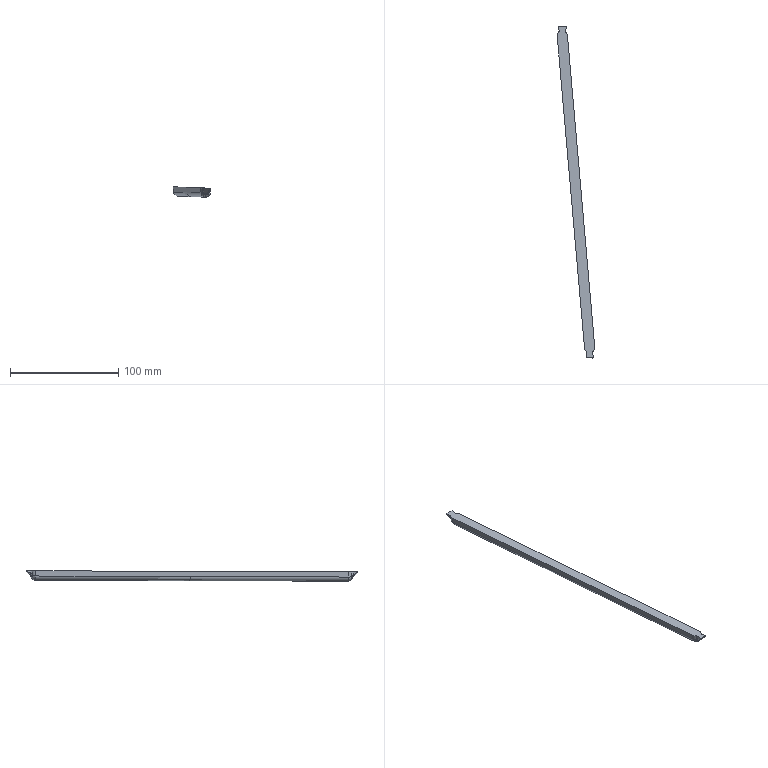Part | Creo | 1 solid | 50 faces | box 34.736 x 306.719 x 9.582 mm | volume 20166 mm3 | spline 28 | plane 12 | cylinder 10 | commonest cylinder face diameters 8.4 x6 8.402 x4